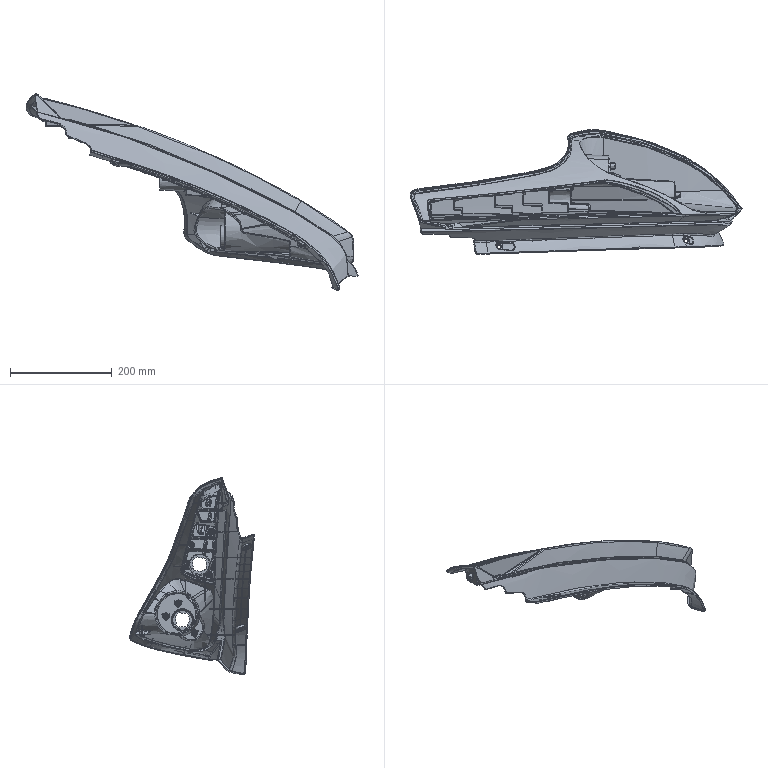Part | STEP file | solid 7 | 1 solid | 1922 faces | box 652.487 x 245.59 x 387.851 mm | volume 665466 mm3 | spline 1415 | plane 222 | sphere 81 | cylinder 78 | cone 61 | torus 55 | other 10 | commonest cylinder face diameters 2.01 x21 4.02 x20 27.135 x8 31.155 x8 2.915 x7 1.005 x6